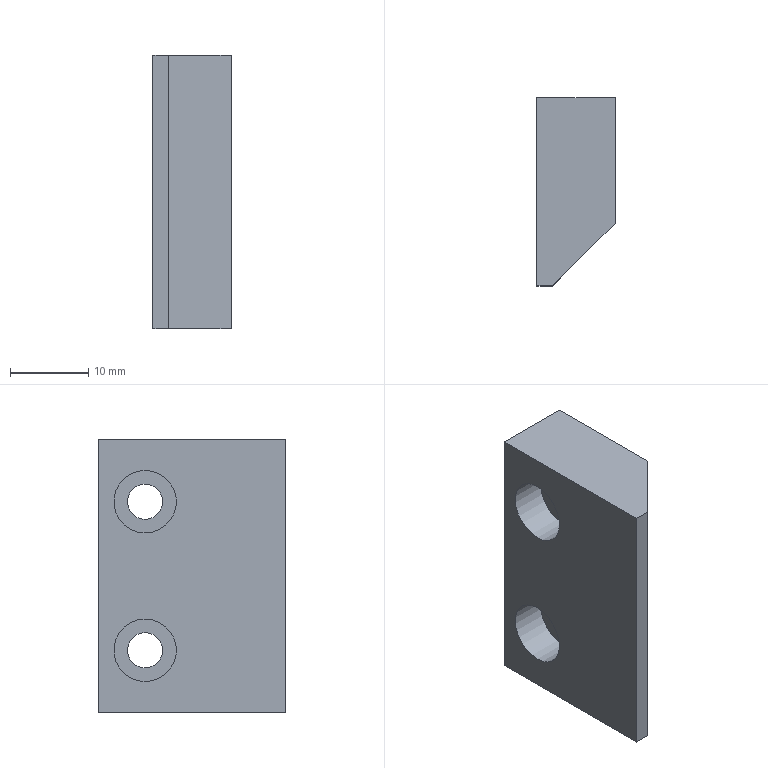Part | NX | 1 solid | 13 faces | box 10 x 24 x 35 mm | volume 6646 mm3 | plane 9 | cylinder 4 | commonest cylinder face diameters 4.5 x2 8 x2
STEP:
#1=CARTESIAN_POINT('',(5.,24.,-174.));
#2=VERTEX_POINT('',#1);
#3=CARTESIAN_POINT('',(5.,8.,-174.));
#4=VERTEX_POINT('',#3);
#5=CARTESIAN_POINT('',(5.,24.,-174.));
#6=DIRECTION('',(0.,-1.,0.));
#7=VECTOR('',#6,1000.);
#8=LINE('',#5,#7);
#9=EDGE_CURVE('',#2,#4,#8,.T.);
#10=ORIENTED_EDGE('',*,*,#9,.T.);
#11=CARTESIAN_POINT('',(-3.,0.,-174.));
#12=VERTEX_POINT('',#11);
#13=CARTESIAN_POINT('',(5.,8.,-174.));
#14=DIRECTION('',(-0.7071,-0.7071,0.));
#15=VECTOR('',#14,1000.);
#16=LINE('',#13,#15);
#17=EDGE_CURVE('',#4,#12,#16,.T.);
#18=ORIENTED_EDGE('',*,*,#17,.T.);
#19=CARTESIAN_POINT('',(-5.,0.,-174.));
#20=VERTEX_POINT('',#19);
#21=CARTESIAN_POINT('',(-5.,0.,-174.));
#22=DIRECTION('',(-1.,0.,0.));
#23=VECTOR('',#22,1000.);
#24=LINE('',#21,#23);
#25=EDGE_CURVE('',#12,#20,#24,.T.);
#26=ORIENTED_EDGE('',*,*,#25,.T.);
#27=CARTESIAN_POINT('',(-5.,24.,-174.));
#28=VERTEX_POINT('',#27);
#29=CARTESIAN_POINT('',(-5.,24.,-174.));
#30=DIRECTION('',(0.,-1.,0.));
#31=VECTOR('',#30,1000.);
#32=LINE('',#29,#31);
#33=EDGE_CURVE('',#28,#20,#32,.T.);
#34=ORIENTED_EDGE('',*,*,#33,.F.);
#35=CARTESIAN_POINT('',(-5.,24.,-174.));
#36=DIRECTION('',(-1.,0.,0.));
#37=VECTOR('',#36,1000.);
#38=LINE('',#35,#37);
#39=EDGE_CURVE('',#2,#28,#38,.T.);
#40=ORIENTED_EDGE('',*,*,#39,.F.);
#41=EDGE_LOOP('',(#10,#18,#26,#34,#40));
#42=FACE_BOUND('',#41,.T.);
#43=CARTESIAN_POINT('',(-5.,24.,-174.));
#44=DIRECTION('',(0.,0.,1.));
#45=DIRECTION('',(1.,0.,0.));
#46=AXIS2_PLACEMENT_3D('',#43,#44,#45);
#47=PLANE('',#46);
#48=ADVANCED_FACE('',(#42),#47,.F.);
#49=CARTESIAN_POINT('',(-5.,24.,-139.));
#50=VERTEX_POINT('',#49);
#51=CARTESIAN_POINT('',(-5.,24.,174.));
#52=DIRECTION('',(0.,0.,1.));
#53=VECTOR('',#52,1000.);
#54=LINE('',#51,#53);
#55=EDGE_CURVE('',#28,#50,#54,.T.);
#56=ORIENTED_EDGE('',*,*,#55,.T.);
#57=CARTESIAN_POINT('',(5.,24.,-139.));
#58=VERTEX_POINT('',#57);
#59=CARTESIAN_POINT('',(5.,24.,-139.));
#60=DIRECTION('',(-1.,0.,0.));
#61=VECTOR('',#60,1000.);
#62=LINE('',#59,#61);
#63=EDGE_CURVE('',#58,#50,#62,.T.);
#64=ORIENTED_EDGE('',*,*,#63,.F.);
#65=CARTESIAN_POINT('',(5.,24.,174.));
#66=DIRECTION('',(0.,0.,-1.));
#67=VECTOR('',#66,1000.);
#68=LINE('',#65,#67);
#69=EDGE_CURVE('',#58,#2,#68,.T.);
#70=ORIENTED_EDGE('',*,*,#69,.T.);
#71=ORIENTED_EDGE('',*,*,#39,.T.);
#72=EDGE_LOOP('',(#56,#64,#70,#71));
#73=FACE_BOUND('',#72,.T.);
#74=CARTESIAN_POINT('',(0.,24.,0.));
#75=DIRECTION('',(0.,-1.,0.));
#76=DIRECTION('',(0.,0.,-1.));
#77=AXIS2_PLACEMENT_3D('',#74,#75,#76);
#78=PLANE('',#77);
#79=ADVANCED_FACE('',(#73),#78,.F.);
#80=CARTESIAN_POINT('',(-3.,0.,-139.));
#81=VERTEX_POINT('',#80);
#82=CARTESIAN_POINT('',(-5.,0.,-139.));
#83=VERTEX_POINT('',#82);
#84=CARTESIAN_POINT('',(5.,0.,-139.));
#85=DIRECTION('',(-1.,0.,0.));
#86=VECTOR('',#85,1000.);
#87=LINE('',#84,#86);
#88=EDGE_CURVE('',#81,#83,#87,.T.);
#89=ORIENTED_EDGE('',*,*,#88,.T.);
#90=CARTESIAN_POINT('',(-5.,0.,174.));
#91=DIRECTION('',(0.,0.,1.));
#92=VECTOR('',#91,1000.);
#93=LINE('',#90,#92);
#94=EDGE_CURVE('',#20,#83,#93,.T.);
#95=ORIENTED_EDGE('',*,*,#94,.F.);
#96=ORIENTED_EDGE('',*,*,#25,.F.);
#97=CARTESIAN_POINT('',(-3.,0.,174.));
#98=DIRECTION('',(0.,0.,1.));
#99=VECTOR('',#98,1000.);
#100=LINE('',#97,#99);
#101=EDGE_CURVE('',#12,#81,#100,.T.);
#102=ORIENTED_EDGE('',*,*,#101,.T.);
#103=EDGE_LOOP('',(#89,#95,#96,#102));
#104=FACE_BOUND('',#103,.T.);
#105=CARTESIAN_POINT('',(0.,0.,0.));
#106=DIRECTION('',(0.,-1.,0.));
#107=DIRECTION('',(0.,0.,-1.));
#108=AXIS2_PLACEMENT_3D('',#105,#106,#107);
#109=PLANE('',#108);
#110=ADVANCED_FACE('',(#104),#109,.T.);
#111=CARTESIAN_POINT('',(5.,8.,-139.));
#112=VERTEX_POINT('',#111);
#113=CARTESIAN_POINT('',(5.,8.,-139.));
#114=DIRECTION('',(0.7071,0.7071,0.));
#115=VECTOR('',#114,1000.);
#116=LINE('',#113,#115);
#117=EDGE_CURVE('',#81,#112,#116,.T.);
#118=ORIENTED_EDGE('',*,*,#117,.F.);
#119=ORIENTED_EDGE('',*,*,#101,.F.);
#120=ORIENTED_EDGE('',*,*,#17,.F.);
#121=CARTESIAN_POINT('',(5.,8.,-174.));
#122=DIRECTION('',(0.,0.,-1.));
#123=VECTOR('',#122,1000.);
#124=LINE('',#121,#123);
#125=EDGE_CURVE('',#112,#4,#124,.T.);
#126=ORIENTED_EDGE('',*,*,#125,.F.);
#127=EDGE_LOOP('',(#118,#119,#120,#126));
#128=FACE_BOUND('',#127,.T.);
#129=CARTESIAN_POINT('',(5.,8.,174.));
#130=DIRECTION('',(0.7071,-0.7071,0.));
#131=DIRECTION('',(0.,0.,1.));
#132=AXIS2_PLACEMENT_3D('',#129,#130,#131);
#133=PLANE('',#132);
#134=ADVANCED_FACE('',(#128),#133,.T.);
#135=CARTESIAN_POINT('',(-5.,18.,-143.));
#136=VERTEX_POINT('',#135);
#137=CARTESIAN_POINT('',(-5.,18.,-147.));
#138=DIRECTION('',(-1.,0.,0.));
#139=DIRECTION('',(0.,0.,1.));
#140=AXIS2_PLACEMENT_3D('',#137,#138,#139);
#141=CIRCLE('',#140,4.);
#142=EDGE_CURVE('',#136,#136,#141,.T.);
#143=ORIENTED_EDGE('',*,*,#142,.F.);
#144=EDGE_LOOP('',(#143));
#145=FACE_BOUND('',#144,.T.);
#146=CARTESIAN_POINT('',(-5.,18.,-162.));
#147=VERTEX_POINT('',#146);
#148=CARTESIAN_POINT('',(-5.,18.,-166.));
#149=DIRECTION('',(-1.,0.,0.));
#150=DIRECTION('',(0.,0.,1.));
#151=AXIS2_PLACEMENT_3D('',#148,#149,#150);
#152=CIRCLE('',#151,4.);
#153=EDGE_CURVE('',#147,#147,#152,.T.);
#154=ORIENTED_EDGE('',*,*,#153,.F.);
#155=EDGE_LOOP('',(#154));
#156=FACE_BOUND('',#155,.T.);
#157=ORIENTED_EDGE('',*,*,#94,.T.);
#158=CARTESIAN_POINT('',(-5.,24.,-139.));
#159=DIRECTION('',(0.,-1.,0.));
#160=VECTOR('',#159,1000.);
#161=LINE('',#158,#160);
#162=EDGE_CURVE('',#50,#83,#161,.T.);
#163=ORIENTED_EDGE('',*,*,#162,.F.);
#164=ORIENTED_EDGE('',*,*,#55,.F.);
#165=ORIENTED_EDGE('',*,*,#33,.T.);
#166=EDGE_LOOP('',(#157,#163,#164,#165));
#167=FACE_BOUND('',#166,.T.);
#168=CARTESIAN_POINT('',(-5.,24.,174.));
#169=DIRECTION('',(1.,0.,0.));
#170=DIRECTION('',(0.,0.,-1.));
#171=AXIS2_PLACEMENT_3D('',#168,#169,#170);
#172=PLANE('',#171);
#173=ADVANCED_FACE('',(#145,#156,#167),#172,.F.);
#174=CARTESIAN_POINT('',(5.,18.,-144.75));
#175=VERTEX_POINT('',#174);
#176=CARTESIAN_POINT('',(5.,18.,-147.));
#177=DIRECTION('',(-1.,0.,0.));
#178=DIRECTION('',(0.,0.,1.));
#179=AXIS2_PLACEMENT_3D('',#176,#177,#178);
#180=CIRCLE('',#179,2.25);
#181=EDGE_CURVE('',#175,#175,#180,.T.);
#182=ORIENTED_EDGE('',*,*,#181,.T.);
#183=EDGE_LOOP('',(#182));
#184=FACE_BOUND('',#183,.T.);
#185=CARTESIAN_POINT('',(5.,18.,-163.75));
#186=VERTEX_POINT('',#185);
#187=CARTESIAN_POINT('',(5.,18.,-166.));
#188=DIRECTION('',(-1.,0.,0.));
#189=DIRECTION('',(0.,0.,1.));
#190=AXIS2_PLACEMENT_3D('',#187,#188,#189);
#191=CIRCLE('',#190,2.25);
#192=EDGE_CURVE('',#186,#186,#191,.T.);
#193=ORIENTED_EDGE('',*,*,#192,.T.);
#194=EDGE_LOOP('',(#193));
#195=FACE_BOUND('',#194,.T.);
#196=ORIENTED_EDGE('',*,*,#69,.F.);
#197=CARTESIAN_POINT('',(5.,24.,-139.));
#198=DIRECTION('',(0.,-1.,0.));
#199=VECTOR('',#198,1000.);
#200=LINE('',#197,#199);
#201=EDGE_CURVE('',#58,#112,#200,.T.);
#202=ORIENTED_EDGE('',*,*,#201,.T.);
#203=ORIENTED_EDGE('',*,*,#125,.T.);
#204=ORIENTED_EDGE('',*,*,#9,.F.);
#205=EDGE_LOOP('',(#196,#202,#203,#204));
#206=FACE_BOUND('',#205,.T.);
#207=CARTESIAN_POINT('',(5.,24.,174.));
#208=DIRECTION('',(-1.,0.,0.));
#209=DIRECTION('',(0.,0.,1.));
#210=AXIS2_PLACEMENT_3D('',#207,#208,#209);
#211=PLANE('',#210);
#212=ADVANCED_FACE('',(#184,#195,#206),#211,.F.);
#213=ORIENTED_EDGE('',*,*,#117,.T.);
#214=ORIENTED_EDGE('',*,*,#201,.F.);
#215=ORIENTED_EDGE('',*,*,#63,.T.);
#216=ORIENTED_EDGE('',*,*,#162,.T.);
#217=ORIENTED_EDGE('',*,*,#88,.F.);
#218=EDGE_LOOP('',(#213,#214,#215,#216,#217));
#219=FACE_BOUND('',#218,.T.);
#220=CARTESIAN_POINT('',(5.,24.,-139.));
#221=DIRECTION('',(0.,0.,-1.));
#222=DIRECTION('',(-1.,0.,0.));
#223=AXIS2_PLACEMENT_3D('',#220,#221,#222);
#224=PLANE('',#223);
#225=ADVANCED_FACE('',(#219),#224,.F.);
#226=ORIENTED_EDGE('',*,*,#192,.F.);
#227=EDGE_LOOP('',(#226));
#228=FACE_BOUND('',#227,.T.);
#229=CARTESIAN_POINT('',(-0.4,18.,-163.75));
#230=VERTEX_POINT('',#229);
#231=CARTESIAN_POINT('',(-0.4,18.,-166.));
#232=DIRECTION('',(-1.,0.,0.));
#233=DIRECTION('',(0.,0.,1.));
#234=AXIS2_PLACEMENT_3D('',#231,#232,#233);
#235=CIRCLE('',#234,2.25);
#236=EDGE_CURVE('',#230,#230,#235,.T.);
#237=ORIENTED_EDGE('',*,*,#236,.T.);
#238=EDGE_LOOP('',(#237));
#239=FACE_BOUND('',#238,.T.);
#240=CARTESIAN_POINT('',(-5.,18.,-166.));
#241=DIRECTION('',(-1.,0.,0.));
#242=DIRECTION('',(0.,0.,1.));
#243=AXIS2_PLACEMENT_3D('',#240,#241,#242);
#244=CYLINDRICAL_SURFACE('',#243,2.25);
#245=ADVANCED_FACE('',(#228,#239),#244,.F.);
#246=ORIENTED_EDGE('',*,*,#236,.F.);
#247=EDGE_LOOP('',(#246));
#248=FACE_BOUND('',#247,.T.);
#249=CARTESIAN_POINT('',(-0.4,18.,-162.));
#250=VERTEX_POINT('',#249);
#251=CARTESIAN_POINT('',(-0.4,18.,-166.));
#252=DIRECTION('',(-1.,0.,0.));
#253=DIRECTION('',(0.,0.,1.));
#254=AXIS2_PLACEMENT_3D('',#251,#252,#253);
#255=CIRCLE('',#254,4.);
#256=EDGE_CURVE('',#250,#250,#255,.T.);
#257=ORIENTED_EDGE('',*,*,#256,.T.);
#258=EDGE_LOOP('',(#257));
#259=FACE_BOUND('',#258,.T.);
#260=CARTESIAN_POINT('',(-0.4,20.25,-166.));
#261=DIRECTION('',(1.,0.,0.));
#262=DIRECTION('',(0.,0.,-1.));
#263=AXIS2_PLACEMENT_3D('',#260,#261,#262);
#264=PLANE('',#263);
#265=ADVANCED_FACE('',(#248,#259),#264,.F.);
#266=ORIENTED_EDGE('',*,*,#256,.F.);
#267=EDGE_LOOP('',(#266));
#268=FACE_BOUND('',#267,.T.);
#269=ORIENTED_EDGE('',*,*,#153,.T.);
#270=EDGE_LOOP('',(#269));
#271=FACE_BOUND('',#270,.T.);
#272=CARTESIAN_POINT('',(-5.,18.,-166.));
#273=DIRECTION('',(-1.,0.,0.));
#274=DIRECTION('',(0.,0.,1.));
#275=AXIS2_PLACEMENT_3D('',#272,#273,#274);
#276=CYLINDRICAL_SURFACE('',#275,4.);
#277=ADVANCED_FACE('',(#268,#271),#276,.F.);
#278=ORIENTED_EDGE('',*,*,#181,.F.);
#279=EDGE_LOOP('',(#278));
#280=FACE_BOUND('',#279,.T.);
#281=CARTESIAN_POINT('',(-0.4,18.,-144.75));
#282=VERTEX_POINT('',#281);
#283=CARTESIAN_POINT('',(-0.4,18.,-147.));
#284=DIRECTION('',(-1.,0.,0.));
#285=DIRECTION('',(0.,0.,1.));
#286=AXIS2_PLACEMENT_3D('',#283,#284,#285);
#287=CIRCLE('',#286,2.25);
#288=EDGE_CURVE('',#282,#282,#287,.T.);
#289=ORIENTED_EDGE('',*,*,#288,.T.);
#290=EDGE_LOOP('',(#289));
#291=FACE_BOUND('',#290,.T.);
#292=CARTESIAN_POINT('',(-5.,18.,-147.));
#293=DIRECTION('',(-1.,0.,0.));
#294=DIRECTION('',(0.,0.,1.));
#295=AXIS2_PLACEMENT_3D('',#292,#293,#294);
#296=CYLINDRICAL_SURFACE('',#295,2.25);
#297=ADVANCED_FACE('',(#280,#291),#296,.F.);
#298=ORIENTED_EDGE('',*,*,#288,.F.);
#299=EDGE_LOOP('',(#298));
#300=FACE_BOUND('',#299,.T.);
#301=CARTESIAN_POINT('',(-0.4,18.,-143.));
#302=VERTEX_POINT('',#301);
#303=CARTESIAN_POINT('',(-0.4,18.,-147.));
#304=DIRECTION('',(-1.,0.,0.));
#305=DIRECTION('',(0.,0.,1.));
#306=AXIS2_PLACEMENT_3D('',#303,#304,#305);
#307=CIRCLE('',#306,4.);
#308=EDGE_CURVE('',#302,#302,#307,.T.);
#309=ORIENTED_EDGE('',*,*,#308,.T.);
#310=EDGE_LOOP('',(#309));
#311=FACE_BOUND('',#310,.T.);
#312=CARTESIAN_POINT('',(-0.4,20.25,-147.));
#313=DIRECTION('',(1.,0.,0.));
#314=DIRECTION('',(0.,0.,-1.));
#315=AXIS2_PLACEMENT_3D('',#312,#313,#314);
#316=PLANE('',#315);
#317=ADVANCED_FACE('',(#300,#311),#316,.F.);
#318=ORIENTED_EDGE('',*,*,#308,.F.);
#319=EDGE_LOOP('',(#318));
#320=FACE_BOUND('',#319,.T.);
#321=ORIENTED_EDGE('',*,*,#142,.T.);
#322=EDGE_LOOP('',(#321));
#323=FACE_BOUND('',#322,.T.);
#324=CARTESIAN_POINT('',(-5.,18.,-147.));
#325=DIRECTION('',(-1.,0.,0.));
#326=DIRECTION('',(0.,0.,1.));
#327=AXIS2_PLACEMENT_3D('',#324,#325,#326);
#328=CYLINDRICAL_SURFACE('',#327,4.);
#329=ADVANCED_FACE('',(#320,#323),#328,.F.);
#330=CLOSED_SHELL('',(#48,#79,#110,#134,#173,#212,#225,#245,#265,#277,#297,#317,#329));
#331=MANIFOLD_SOLID_BREP('',#330);
#332=(LENGTH_UNIT()NAMED_UNIT(*)SI_UNIT(.MILLI.,.METRE.));
#333=UNCERTAINTY_MEASURE_WITH_UNIT(LENGTH_MEASURE(0.00001),#332,'','');
#334=(NAMED_UNIT(*)PLANE_ANGLE_UNIT()SI_UNIT($,.RADIAN.));
#335=(NAMED_UNIT(*)SI_UNIT($,.STERADIAN.)SOLID_ANGLE_UNIT());
#336=(GEOMETRIC_REPRESENTATION_CONTEXT(3)GLOBAL_UNCERTAINTY_ASSIGNED_CONTEXT((#333))GLOBAL_UNIT_ASSIGNED_CONTEXT((#332,#334,#335))REPRESENTATION_CONTEXT('',''));
#337=ADVANCED_BREP_SHAPE_REPRESENTATION('',(#331),#336);